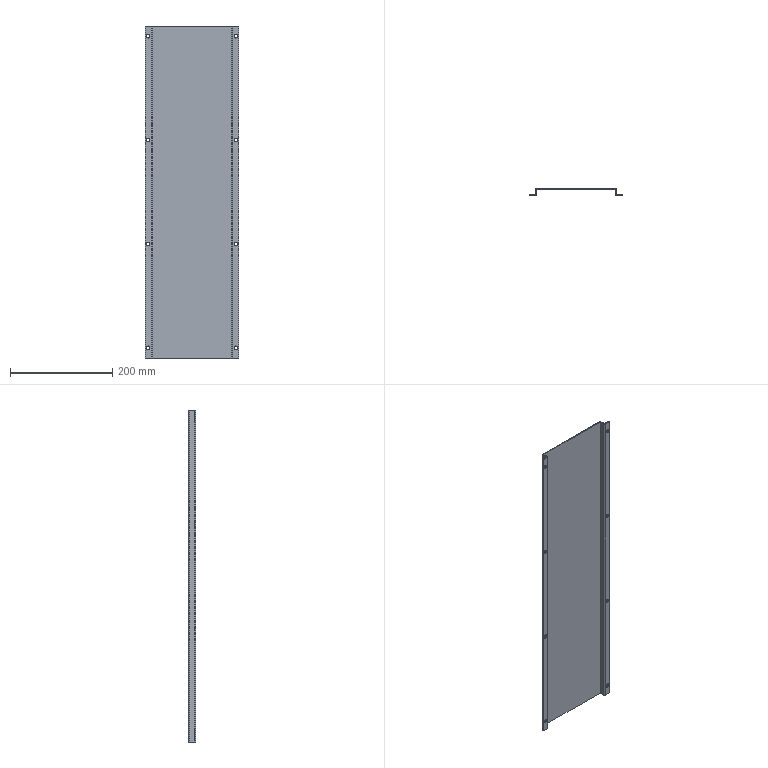Part | STEP file | Brake Resistor Plate | 1 solid | 38 faces | box 184 x 14 x 650 mm | volume 267329 mm3 | cylinder 24 | plane 14 | commonest cylinder face diameters 7 x16 0.2 x4 4.2 x4
STEP:
#1=CARTESIAN_POINT('',(61.034,19.025,633.5));
#2=VERTEX_POINT('',#1);
#3=CARTESIAN_POINT('',(61.034,19.025,626.5));
#4=VERTEX_POINT('',#3);
#5=CARTESIAN_POINT('',(61.034,19.025,630.));
#6=DIRECTION('',(0.,-1.,0.));
#7=DIRECTION('',(0.,0.,1.));
#8=AXIS2_PLACEMENT_3D('',#5,#6,#7);
#9=CIRCLE('',#8,3.5);
#10=EDGE_CURVE('',#2,#4,#9,.T.);
#11=ORIENTED_EDGE('',*,*,#10,.T.);
#12=CARTESIAN_POINT('',(61.034,21.025,626.5));
#13=VERTEX_POINT('',#12);
#14=CARTESIAN_POINT('',(61.034,11.025,626.5));
#15=DIRECTION('',(0.,1.,0.));
#16=VECTOR('',#15,1000.);
#17=LINE('',#14,#16);
#18=EDGE_CURVE('',#4,#13,#17,.T.);
#19=ORIENTED_EDGE('',*,*,#18,.T.);
#20=CARTESIAN_POINT('',(61.034,21.025,633.5));
#21=VERTEX_POINT('',#20);
#22=CARTESIAN_POINT('',(61.034,21.025,630.));
#23=DIRECTION('',(0.,-1.,0.));
#24=DIRECTION('',(0.,0.,1.));
#25=AXIS2_PLACEMENT_3D('',#22,#23,#24);
#26=CIRCLE('',#25,3.5);
#27=EDGE_CURVE('',#21,#13,#26,.T.);
#28=ORIENTED_EDGE('',*,*,#27,.F.);
#29=CARTESIAN_POINT('',(61.034,11.025,633.5));
#30=DIRECTION('',(0.,1.,0.));
#31=VECTOR('',#30,1000.);
#32=LINE('',#29,#31);
#33=EDGE_CURVE('',#2,#21,#32,.T.);
#34=ORIENTED_EDGE('',*,*,#33,.F.);
#35=EDGE_LOOP('',(#11,#19,#28,#34));
#36=FACE_OUTER_BOUND('',#35,.T.);
#37=CARTESIAN_POINT('',(61.034,11.025,630.));
#38=DIRECTION('',(0.,1.,0.));
#39=DIRECTION('',(0.,0.,1.));
#40=AXIS2_PLACEMENT_3D('',#37,#38,#39);
#41=CYLINDRICAL_SURFACE('',#40,3.5);
#42=ADVANCED_FACE('',(#36),#41,.F.);
#43=CARTESIAN_POINT('',(61.034,19.025,430.167));
#44=VERTEX_POINT('',#43);
#45=CARTESIAN_POINT('',(61.034,19.025,423.167));
#46=VERTEX_POINT('',#45);
#47=CARTESIAN_POINT('',(61.034,19.025,426.667));
#48=DIRECTION('',(0.,-1.,0.));
#49=DIRECTION('',(0.,0.,1.));
#50=AXIS2_PLACEMENT_3D('',#47,#48,#49);
#51=CIRCLE('',#50,3.5);
#52=EDGE_CURVE('',#44,#46,#51,.T.);
#53=ORIENTED_EDGE('',*,*,#52,.T.);
#54=CARTESIAN_POINT('',(61.034,21.025,423.167));
#55=VERTEX_POINT('',#54);
#56=CARTESIAN_POINT('',(61.034,11.025,423.167));
#57=DIRECTION('',(0.,1.,0.));
#58=VECTOR('',#57,1000.);
#59=LINE('',#56,#58);
#60=EDGE_CURVE('',#46,#55,#59,.T.);
#61=ORIENTED_EDGE('',*,*,#60,.T.);
#62=CARTESIAN_POINT('',(61.034,21.025,430.167));
#63=VERTEX_POINT('',#62);
#64=CARTESIAN_POINT('',(61.034,21.025,426.667));
#65=DIRECTION('',(0.,-1.,0.));
#66=DIRECTION('',(0.,0.,1.));
#67=AXIS2_PLACEMENT_3D('',#64,#65,#66);
#68=CIRCLE('',#67,3.5);
#69=EDGE_CURVE('',#63,#55,#68,.T.);
#70=ORIENTED_EDGE('',*,*,#69,.F.);
#71=CARTESIAN_POINT('',(61.034,11.025,430.167));
#72=DIRECTION('',(0.,1.,0.));
#73=VECTOR('',#72,1000.);
#74=LINE('',#71,#73);
#75=EDGE_CURVE('',#44,#63,#74,.T.);
#76=ORIENTED_EDGE('',*,*,#75,.F.);
#77=EDGE_LOOP('',(#53,#61,#70,#76));
#78=FACE_OUTER_BOUND('',#77,.T.);
#79=CARTESIAN_POINT('',(61.034,11.025,426.667));
#80=DIRECTION('',(0.,1.,0.));
#81=DIRECTION('',(0.,0.,1.));
#82=AXIS2_PLACEMENT_3D('',#79,#80,#81);
#83=CYLINDRICAL_SURFACE('',#82,3.5);
#84=ADVANCED_FACE('',(#78),#83,.F.);
#85=CARTESIAN_POINT('',(61.034,19.025,226.833));
#86=VERTEX_POINT('',#85);
#87=CARTESIAN_POINT('',(61.034,19.025,219.833));
#88=VERTEX_POINT('',#87);
#89=CARTESIAN_POINT('',(61.034,19.025,223.333));
#90=DIRECTION('',(0.,-1.,0.));
#91=DIRECTION('',(0.,0.,1.));
#92=AXIS2_PLACEMENT_3D('',#89,#90,#91);
#93=CIRCLE('',#92,3.5);
#94=EDGE_CURVE('',#86,#88,#93,.T.);
#95=ORIENTED_EDGE('',*,*,#94,.T.);
#96=CARTESIAN_POINT('',(61.034,21.025,219.833));
#97=VERTEX_POINT('',#96);
#98=CARTESIAN_POINT('',(61.034,11.025,219.833));
#99=DIRECTION('',(0.,1.,0.));
#100=VECTOR('',#99,1000.);
#101=LINE('',#98,#100);
#102=EDGE_CURVE('',#88,#97,#101,.T.);
#103=ORIENTED_EDGE('',*,*,#102,.T.);
#104=CARTESIAN_POINT('',(61.034,21.025,226.833));
#105=VERTEX_POINT('',#104);
#106=CARTESIAN_POINT('',(61.034,21.025,223.333));
#107=DIRECTION('',(0.,-1.,0.));
#108=DIRECTION('',(0.,0.,1.));
#109=AXIS2_PLACEMENT_3D('',#106,#107,#108);
#110=CIRCLE('',#109,3.5);
#111=EDGE_CURVE('',#105,#97,#110,.T.);
#112=ORIENTED_EDGE('',*,*,#111,.F.);
#113=CARTESIAN_POINT('',(61.034,11.025,226.833));
#114=DIRECTION('',(0.,1.,0.));
#115=VECTOR('',#114,1000.);
#116=LINE('',#113,#115);
#117=EDGE_CURVE('',#86,#105,#116,.T.);
#118=ORIENTED_EDGE('',*,*,#117,.F.);
#119=EDGE_LOOP('',(#95,#103,#112,#118));
#120=FACE_OUTER_BOUND('',#119,.T.);
#121=CARTESIAN_POINT('',(61.034,11.025,223.333));
#122=DIRECTION('',(0.,1.,0.));
#123=DIRECTION('',(0.,0.,1.));
#124=AXIS2_PLACEMENT_3D('',#121,#122,#123);
#125=CYLINDRICAL_SURFACE('',#124,3.5);
#126=ADVANCED_FACE('',(#120),#125,.F.);
#127=CARTESIAN_POINT('',(61.034,19.025,23.5));
#128=VERTEX_POINT('',#127);
#129=CARTESIAN_POINT('',(61.034,19.025,16.5));
#130=VERTEX_POINT('',#129);
#131=CARTESIAN_POINT('',(61.034,19.025,20.));
#132=DIRECTION('',(0.,-1.,0.));
#133=DIRECTION('',(0.,0.,1.));
#134=AXIS2_PLACEMENT_3D('',#131,#132,#133);
#135=CIRCLE('',#134,3.5);
#136=EDGE_CURVE('',#128,#130,#135,.T.);
#137=ORIENTED_EDGE('',*,*,#136,.T.);
#138=CARTESIAN_POINT('',(61.034,21.025,16.5));
#139=VERTEX_POINT('',#138);
#140=CARTESIAN_POINT('',(61.034,11.025,16.5));
#141=DIRECTION('',(0.,1.,0.));
#142=VECTOR('',#141,1000.);
#143=LINE('',#140,#142);
#144=EDGE_CURVE('',#130,#139,#143,.T.);
#145=ORIENTED_EDGE('',*,*,#144,.T.);
#146=CARTESIAN_POINT('',(61.034,21.025,23.5));
#147=VERTEX_POINT('',#146);
#148=CARTESIAN_POINT('',(61.034,21.025,20.));
#149=DIRECTION('',(0.,-1.,0.));
#150=DIRECTION('',(0.,0.,1.));
#151=AXIS2_PLACEMENT_3D('',#148,#149,#150);
#152=CIRCLE('',#151,3.5);
#153=EDGE_CURVE('',#147,#139,#152,.T.);
#154=ORIENTED_EDGE('',*,*,#153,.F.);
#155=CARTESIAN_POINT('',(61.034,11.025,23.5));
#156=DIRECTION('',(0.,1.,0.));
#157=VECTOR('',#156,1000.);
#158=LINE('',#155,#157);
#159=EDGE_CURVE('',#128,#147,#158,.T.);
#160=ORIENTED_EDGE('',*,*,#159,.F.);
#161=EDGE_LOOP('',(#137,#145,#154,#160));
#162=FACE_OUTER_BOUND('',#161,.T.);
#163=CARTESIAN_POINT('',(61.034,11.025,20.));
#164=DIRECTION('',(0.,1.,0.));
#165=DIRECTION('',(0.,0.,1.));
#166=AXIS2_PLACEMENT_3D('',#163,#164,#165);
#167=CYLINDRICAL_SURFACE('',#166,3.5);
#168=ADVANCED_FACE('',(#162),#167,.F.);
#169=CARTESIAN_POINT('',(-111.015,19.025,633.5));
#170=VERTEX_POINT('',#169);
#171=CARTESIAN_POINT('',(-111.015,19.025,626.5));
#172=VERTEX_POINT('',#171);
#173=CARTESIAN_POINT('',(-111.015,19.025,630.));
#174=DIRECTION('',(0.,-1.,0.));
#175=DIRECTION('',(0.,0.,1.));
#176=AXIS2_PLACEMENT_3D('',#173,#174,#175);
#177=CIRCLE('',#176,3.5);
#178=EDGE_CURVE('',#170,#172,#177,.T.);
#179=ORIENTED_EDGE('',*,*,#178,.T.);
#180=CARTESIAN_POINT('',(-111.015,21.025,626.5));
#181=VERTEX_POINT('',#180);
#182=CARTESIAN_POINT('',(-111.015,11.025,626.5));
#183=DIRECTION('',(0.,1.,0.));
#184=VECTOR('',#183,1000.);
#185=LINE('',#182,#184);
#186=EDGE_CURVE('',#172,#181,#185,.T.);
#187=ORIENTED_EDGE('',*,*,#186,.T.);
#188=CARTESIAN_POINT('',(-111.015,21.025,633.5));
#189=VERTEX_POINT('',#188);
#190=CARTESIAN_POINT('',(-111.015,21.025,630.));
#191=DIRECTION('',(0.,-1.,0.));
#192=DIRECTION('',(0.,0.,1.));
#193=AXIS2_PLACEMENT_3D('',#190,#191,#192);
#194=CIRCLE('',#193,3.5);
#195=EDGE_CURVE('',#189,#181,#194,.T.);
#196=ORIENTED_EDGE('',*,*,#195,.F.);
#197=CARTESIAN_POINT('',(-111.015,11.025,633.5));
#198=DIRECTION('',(0.,1.,0.));
#199=VECTOR('',#198,1000.);
#200=LINE('',#197,#199);
#201=EDGE_CURVE('',#170,#189,#200,.T.);
#202=ORIENTED_EDGE('',*,*,#201,.F.);
#203=EDGE_LOOP('',(#179,#187,#196,#202));
#204=FACE_OUTER_BOUND('',#203,.T.);
#205=CARTESIAN_POINT('',(-111.015,11.025,630.));
#206=DIRECTION('',(0.,1.,0.));
#207=DIRECTION('',(0.,0.,1.));
#208=AXIS2_PLACEMENT_3D('',#205,#206,#207);
#209=CYLINDRICAL_SURFACE('',#208,3.5);
#210=ADVANCED_FACE('',(#204),#209,.F.);
#211=CARTESIAN_POINT('',(-111.015,19.025,430.167));
#212=VERTEX_POINT('',#211);
#213=CARTESIAN_POINT('',(-111.015,19.025,423.167));
#214=VERTEX_POINT('',#213);
#215=CARTESIAN_POINT('',(-111.015,19.025,426.667));
#216=DIRECTION('',(0.,-1.,0.));
#217=DIRECTION('',(0.,0.,1.));
#218=AXIS2_PLACEMENT_3D('',#215,#216,#217);
#219=CIRCLE('',#218,3.5);
#220=EDGE_CURVE('',#212,#214,#219,.T.);
#221=ORIENTED_EDGE('',*,*,#220,.T.);
#222=CARTESIAN_POINT('',(-111.015,21.025,423.167));
#223=VERTEX_POINT('',#222);
#224=CARTESIAN_POINT('',(-111.015,11.025,423.167));
#225=DIRECTION('',(0.,1.,0.));
#226=VECTOR('',#225,1000.);
#227=LINE('',#224,#226);
#228=EDGE_CURVE('',#214,#223,#227,.T.);
#229=ORIENTED_EDGE('',*,*,#228,.T.);
#230=CARTESIAN_POINT('',(-111.015,21.025,430.167));
#231=VERTEX_POINT('',#230);
#232=CARTESIAN_POINT('',(-111.015,21.025,426.667));
#233=DIRECTION('',(0.,-1.,0.));
#234=DIRECTION('',(0.,0.,1.));
#235=AXIS2_PLACEMENT_3D('',#232,#233,#234);
#236=CIRCLE('',#235,3.5);
#237=EDGE_CURVE('',#231,#223,#236,.T.);
#238=ORIENTED_EDGE('',*,*,#237,.F.);
#239=CARTESIAN_POINT('',(-111.015,11.025,430.167));
#240=DIRECTION('',(0.,1.,0.));
#241=VECTOR('',#240,1000.);
#242=LINE('',#239,#241);
#243=EDGE_CURVE('',#212,#231,#242,.T.);
#244=ORIENTED_EDGE('',*,*,#243,.F.);
#245=EDGE_LOOP('',(#221,#229,#238,#244));
#246=FACE_OUTER_BOUND('',#245,.T.);
#247=CARTESIAN_POINT('',(-111.015,11.025,426.667));
#248=DIRECTION('',(0.,1.,0.));
#249=DIRECTION('',(0.,0.,1.));
#250=AXIS2_PLACEMENT_3D('',#247,#248,#249);
#251=CYLINDRICAL_SURFACE('',#250,3.5);
#252=ADVANCED_FACE('',(#246),#251,.F.);
#253=CARTESIAN_POINT('',(-111.015,19.025,226.833));
#254=VERTEX_POINT('',#253);
#255=CARTESIAN_POINT('',(-111.015,19.025,219.833));
#256=VERTEX_POINT('',#255);
#257=CARTESIAN_POINT('',(-111.015,19.025,223.333));
#258=DIRECTION('',(0.,-1.,0.));
#259=DIRECTION('',(0.,0.,1.));
#260=AXIS2_PLACEMENT_3D('',#257,#258,#259);
#261=CIRCLE('',#260,3.5);
#262=EDGE_CURVE('',#254,#256,#261,.T.);
#263=ORIENTED_EDGE('',*,*,#262,.T.);
#264=CARTESIAN_POINT('',(-111.015,21.025,219.833));
#265=VERTEX_POINT('',#264);
#266=CARTESIAN_POINT('',(-111.015,11.025,219.833));
#267=DIRECTION('',(0.,1.,0.));
#268=VECTOR('',#267,1000.);
#269=LINE('',#266,#268);
#270=EDGE_CURVE('',#256,#265,#269,.T.);
#271=ORIENTED_EDGE('',*,*,#270,.T.);
#272=CARTESIAN_POINT('',(-111.015,21.025,226.833));
#273=VERTEX_POINT('',#272);
#274=CARTESIAN_POINT('',(-111.015,21.025,223.333));
#275=DIRECTION('',(0.,-1.,0.));
#276=DIRECTION('',(0.,0.,1.));
#277=AXIS2_PLACEMENT_3D('',#274,#275,#276);
#278=CIRCLE('',#277,3.5);
#279=EDGE_CURVE('',#273,#265,#278,.T.);
#280=ORIENTED_EDGE('',*,*,#279,.F.);
#281=CARTESIAN_POINT('',(-111.015,11.025,226.833));
#282=DIRECTION('',(0.,1.,0.));
#283=VECTOR('',#282,1000.);
#284=LINE('',#281,#283);
#285=EDGE_CURVE('',#254,#273,#284,.T.);
#286=ORIENTED_EDGE('',*,*,#285,.F.);
#287=EDGE_LOOP('',(#263,#271,#280,#286));
#288=FACE_OUTER_BOUND('',#287,.T.);
#289=CARTESIAN_POINT('',(-111.015,11.025,223.333));
#290=DIRECTION('',(0.,1.,0.));
#291=DIRECTION('',(0.,0.,1.));
#292=AXIS2_PLACEMENT_3D('',#289,#290,#291);
#293=CYLINDRICAL_SURFACE('',#292,3.5);
#294=ADVANCED_FACE('',(#288),#293,.F.);
#295=CARTESIAN_POINT('',(-111.015,19.025,23.5));
#296=VERTEX_POINT('',#295);
#297=CARTESIAN_POINT('',(-111.015,19.025,16.5));
#298=VERTEX_POINT('',#297);
#299=CARTESIAN_POINT('',(-111.015,19.025,20.));
#300=DIRECTION('',(0.,-1.,0.));
#301=DIRECTION('',(0.,0.,1.));
#302=AXIS2_PLACEMENT_3D('',#299,#300,#301);
#303=CIRCLE('',#302,3.5);
#304=EDGE_CURVE('',#296,#298,#303,.T.);
#305=ORIENTED_EDGE('',*,*,#304,.T.);
#306=CARTESIAN_POINT('',(-111.015,21.025,16.5));
#307=VERTEX_POINT('',#306);
#308=CARTESIAN_POINT('',(-111.015,11.025,16.5));
#309=DIRECTION('',(0.,1.,0.));
#310=VECTOR('',#309,1000.);
#311=LINE('',#308,#310);
#312=EDGE_CURVE('',#298,#307,#311,.T.);
#313=ORIENTED_EDGE('',*,*,#312,.T.);
#314=CARTESIAN_POINT('',(-111.015,21.025,23.5));
#315=VERTEX_POINT('',#314);
#316=CARTESIAN_POINT('',(-111.015,21.025,20.));
#317=DIRECTION('',(0.,-1.,0.));
#318=DIRECTION('',(0.,0.,1.));
#319=AXIS2_PLACEMENT_3D('',#316,#317,#318);
#320=CIRCLE('',#319,3.5);
#321=EDGE_CURVE('',#315,#307,#320,.T.);
#322=ORIENTED_EDGE('',*,*,#321,.F.);
#323=CARTESIAN_POINT('',(-111.015,11.025,23.5));
#324=DIRECTION('',(0.,1.,0.));
#325=VECTOR('',#324,1000.);
#326=LINE('',#323,#325);
#327=EDGE_CURVE('',#296,#315,#326,.T.);
#328=ORIENTED_EDGE('',*,*,#327,.F.);
#329=EDGE_LOOP('',(#305,#313,#322,#328));
#330=FACE_OUTER_BOUND('',#329,.T.);
#331=CARTESIAN_POINT('',(-111.015,11.025,20.));
#332=DIRECTION('',(0.,1.,0.));
#333=DIRECTION('',(0.,0.,1.));
#334=AXIS2_PLACEMENT_3D('',#331,#332,#333);
#335=CYLINDRICAL_SURFACE('',#334,3.5);
#336=ADVANCED_FACE('',(#330),#335,.F.);
#337=CARTESIAN_POINT('',(52.934,31.025,650.));
#338=VERTEX_POINT('',#337);
#339=CARTESIAN_POINT('',(52.934,31.025,0.));
#340=VERTEX_POINT('',#339);
#341=CARTESIAN_POINT('',(52.934,31.025,650.));
#342=DIRECTION('',(0.,0.,-1.));
#343=VECTOR('',#342,1000.);
#344=LINE('',#341,#343);
#345=EDGE_CURVE('',#338,#340,#344,.T.);
#346=ORIENTED_EDGE('',*,*,#345,.F.);
#347=CARTESIAN_POINT('',(-102.866,31.025,650.));
#348=VERTEX_POINT('',#347);
#349=CARTESIAN_POINT('',(-104.966,31.025,650.));
#350=DIRECTION('',(1.,0.,0.));
#351=VECTOR('',#350,1000.);
#352=LINE('',#349,#351);
#353=EDGE_CURVE('',#348,#338,#352,.T.);
#354=ORIENTED_EDGE('',*,*,#353,.F.);
#355=CARTESIAN_POINT('',(-102.866,31.025,0.));
#356=VERTEX_POINT('',#355);
#357=CARTESIAN_POINT('',(-102.866,31.025,650.));
#358=DIRECTION('',(0.,0.,1.));
#359=VECTOR('',#358,1000.);
#360=LINE('',#357,#359);
#361=EDGE_CURVE('',#356,#348,#360,.T.);
#362=ORIENTED_EDGE('',*,*,#361,.F.);
#363=CARTESIAN_POINT('',(-104.966,31.025,0.));
#364=DIRECTION('',(-1.,0.,0.));
#365=VECTOR('',#364,1000.);
#366=LINE('',#363,#365);
#367=EDGE_CURVE('',#340,#356,#366,.T.);
#368=ORIENTED_EDGE('',*,*,#367,.F.);
#369=EDGE_LOOP('',(#346,#354,#362,#368));
#370=FACE_OUTER_BOUND('',#369,.T.);
#371=CARTESIAN_POINT('',(-104.966,31.025,650.));
#372=DIRECTION('',(0.,1.,0.));
#373=DIRECTION('',(0.,0.,1.));
#374=AXIS2_PLACEMENT_3D('',#371,#372,#373);
#375=PLANE('',#374);
#376=ADVANCED_FACE('',(#370),#375,.F.);
#377=ORIENTED_EDGE('',*,*,#367,.T.);
#378=CARTESIAN_POINT('',(-102.966,30.925,0.));
#379=VERTEX_POINT('',#378);
#380=CARTESIAN_POINT('',(-102.866,30.925,0.));
#381=DIRECTION('',(0.,0.,1.));
#382=DIRECTION('',(-1.,0.,0.));
#383=AXIS2_PLACEMENT_3D('',#380,#381,#382);
#384=CIRCLE('',#383,0.1);
#385=EDGE_CURVE('',#356,#379,#384,.T.);
#386=ORIENTED_EDGE('',*,*,#385,.T.);
#387=CARTESIAN_POINT('',(-102.966,21.125,0.));
#388=VERTEX_POINT('',#387);
#389=CARTESIAN_POINT('',(-102.966,21.025,0.));
#390=DIRECTION('',(0.,-1.,0.));
#391=VECTOR('',#390,1000.);
#392=LINE('',#389,#391);
#393=EDGE_CURVE('',#379,#388,#392,.T.);
#394=ORIENTED_EDGE('',*,*,#393,.T.);
#395=CARTESIAN_POINT('',(-105.066,19.025,0.));
#396=VERTEX_POINT('',#395);
#397=CARTESIAN_POINT('',(-105.066,21.125,0.));
#398=DIRECTION('',(0.,0.,1.));
#399=DIRECTION('',(-1.,0.,0.));
#400=AXIS2_PLACEMENT_3D('',#397,#398,#399);
#401=CIRCLE('',#400,2.1);
#402=EDGE_CURVE('',#396,#388,#401,.T.);
#403=ORIENTED_EDGE('',*,*,#402,.F.);
#404=CARTESIAN_POINT('',(-116.966,19.025,0.));
#405=VERTEX_POINT('',#404);
#406=CARTESIAN_POINT('',(-116.966,19.025,0.));
#407=DIRECTION('',(-1.,0.,0.));
#408=VECTOR('',#407,1000.);
#409=LINE('',#406,#408);
#410=EDGE_CURVE('',#396,#405,#409,.T.);
#411=ORIENTED_EDGE('',*,*,#410,.T.);
#412=CARTESIAN_POINT('',(-116.966,21.025,0.));
#413=VERTEX_POINT('',#412);
#414=CARTESIAN_POINT('',(-116.966,21.125,0.));
#415=DIRECTION('',(0.,1.,0.));
#416=VECTOR('',#415,1000.);
#417=LINE('',#414,#416);
#418=EDGE_CURVE('',#405,#413,#417,.T.);
#419=ORIENTED_EDGE('',*,*,#418,.T.);
#420=CARTESIAN_POINT('',(-105.066,21.025,0.));
#421=VERTEX_POINT('',#420);
#422=CARTESIAN_POINT('',(-102.966,21.025,0.));
#423=DIRECTION('',(1.,0.,0.));
#424=VECTOR('',#423,1000.);
#425=LINE('',#422,#424);
#426=EDGE_CURVE('',#413,#421,#425,.T.);
#427=ORIENTED_EDGE('',*,*,#426,.T.);
#428=CARTESIAN_POINT('',(-104.966,21.125,0.));
#429=VERTEX_POINT('',#428);
#430=CARTESIAN_POINT('',(-105.066,21.125,0.));
#431=DIRECTION('',(0.,0.,1.));
#432=DIRECTION('',(-1.,0.,0.));
#433=AXIS2_PLACEMENT_3D('',#430,#431,#432);
#434=CIRCLE('',#433,0.1);
#435=EDGE_CURVE('',#421,#429,#434,.T.);
#436=ORIENTED_EDGE('',*,*,#435,.T.);
#437=CARTESIAN_POINT('',(-104.966,30.925,0.));
#438=VERTEX_POINT('',#437);
#439=CARTESIAN_POINT('',(-104.966,31.025,0.));
#440=DIRECTION('',(0.,1.,0.));
#441=VECTOR('',#440,1000.);
#442=LINE('',#439,#441);
#443=EDGE_CURVE('',#429,#438,#442,.T.);
#444=ORIENTED_EDGE('',*,*,#443,.T.);
#445=CARTESIAN_POINT('',(-102.866,33.025,0.));
#446=VERTEX_POINT('',#445);
#447=CARTESIAN_POINT('',(-102.866,30.925,0.));
#448=DIRECTION('',(0.,0.,-1.));
#449=DIRECTION('',(-1.,0.,0.));
#450=AXIS2_PLACEMENT_3D('',#447,#448,#449);
#451=CIRCLE('',#450,2.1);
#452=EDGE_CURVE('',#438,#446,#451,.T.);
#453=ORIENTED_EDGE('',*,*,#452,.T.);
#454=CARTESIAN_POINT('',(52.934,33.025,0.));
#455=VERTEX_POINT('',#454);
#456=CARTESIAN_POINT('',(53.034,33.025,0.));
#457=DIRECTION('',(1.,0.,0.));
#458=VECTOR('',#457,1000.);
#459=LINE('',#456,#458);
#460=EDGE_CURVE('',#446,#455,#459,.T.);
#461=ORIENTED_EDGE('',*,*,#460,.T.);
#462=CARTESIAN_POINT('',(55.034,30.925,0.));
#463=VERTEX_POINT('',#462);
#464=CARTESIAN_POINT('',(52.934,30.925,0.));
#465=DIRECTION('',(0.,0.,-1.));
#466=DIRECTION('',(-1.,0.,0.));
#467=AXIS2_PLACEMENT_3D('',#464,#465,#466);
#468=CIRCLE('',#467,2.1);
#469=EDGE_CURVE('',#455,#463,#468,.T.);
#470=ORIENTED_EDGE('',*,*,#469,.T.);
#471=CARTESIAN_POINT('',(55.034,21.125,0.));
#472=VERTEX_POINT('',#471);
#473=CARTESIAN_POINT('',(55.034,19.025,0.));
#474=DIRECTION('',(0.,-1.,0.));
#475=VECTOR('',#474,1000.);
#476=LINE('',#473,#475);
#477=EDGE_CURVE('',#463,#472,#476,.T.);
#478=ORIENTED_EDGE('',*,*,#477,.T.);
#479=CARTESIAN_POINT('',(55.134,21.025,0.));
#480=VERTEX_POINT('',#479);
#481=CARTESIAN_POINT('',(55.134,21.125,0.));
#482=DIRECTION('',(0.,0.,1.));
#483=DIRECTION('',(-1.,0.,0.));
#484=AXIS2_PLACEMENT_3D('',#481,#482,#483);
#485=CIRCLE('',#484,0.1);
#486=EDGE_CURVE('',#472,#480,#485,.T.);
#487=ORIENTED_EDGE('',*,*,#486,.T.);
#488=CARTESIAN_POINT('',(67.034,21.025,0.));
#489=VERTEX_POINT('',#488);
#490=CARTESIAN_POINT('',(55.134,21.025,0.));
#491=DIRECTION('',(1.,0.,0.));
#492=VECTOR('',#491,1000.);
#493=LINE('',#490,#492);
#494=EDGE_CURVE('',#480,#489,#493,.T.);
#495=ORIENTED_EDGE('',*,*,#494,.T.);
#496=CARTESIAN_POINT('',(67.034,19.025,0.));
#497=VERTEX_POINT('',#496);
#498=CARTESIAN_POINT('',(67.034,21.125,0.));
#499=DIRECTION('',(0.,-1.,0.));
#500=VECTOR('',#499,1000.);
#501=LINE('',#498,#500);
#502=EDGE_CURVE('',#489,#497,#501,.T.);
#503=ORIENTED_EDGE('',*,*,#502,.T.);
#504=CARTESIAN_POINT('',(55.134,19.025,0.));
#505=VERTEX_POINT('',#504);
#506=CARTESIAN_POINT('',(55.034,19.025,0.));
#507=DIRECTION('',(-1.,0.,0.));
#508=VECTOR('',#507,1000.);
#509=LINE('',#506,#508);
#510=EDGE_CURVE('',#497,#505,#509,.T.);
#511=ORIENTED_EDGE('',*,*,#510,.T.);
#512=CARTESIAN_POINT('',(53.034,21.125,0.));
#513=VERTEX_POINT('',#512);
#514=CARTESIAN_POINT('',(55.134,21.125,0.));
#515=DIRECTION('',(0.,0.,1.));
#516=DIRECTION('',(-1.,0.,0.));
#517=AXIS2_PLACEMENT_3D('',#514,#515,#516);
#518=CIRCLE('',#517,2.1);
#519=EDGE_CURVE('',#513,#505,#518,.T.);
#520=ORIENTED_EDGE('',*,*,#519,.F.);
#521=CARTESIAN_POINT('',(53.034,30.925,0.));
#522=VERTEX_POINT('',#521);
#523=CARTESIAN_POINT('',(53.034,33.025,0.));
#524=DIRECTION('',(0.,1.,0.));
#525=VECTOR('',#524,1000.);
#526=LINE('',#523,#525);
#527=EDGE_CURVE('',#513,#522,#526,.T.);
#528=ORIENTED_EDGE('',*,*,#527,.T.);
#529=CARTESIAN_POINT('',(52.934,30.925,0.));
#530=DIRECTION('',(0.,0.,1.));
#531=DIRECTION('',(-1.,0.,0.));
#532=AXIS2_PLACEMENT_3D('',#529,#530,#531);
#533=CIRCLE('',#532,0.1);
#534=EDGE_CURVE('',#522,#340,#533,.T.);
#535=ORIENTED_EDGE('',*,*,#534,.T.);
#536=EDGE_LOOP('',(#377,#386,#394,#403,#411,#419,#427,#436,#444,#453,#461,#470,#478,#487,#495,#503,#511,#520,#528,#535));
#537=FACE_OUTER_BOUND('',#536,.T.);
#538=CARTESIAN_POINT('',(53.034,30.925,0.));
#539=DIRECTION('',(0.,0.,-1.));
#540=DIRECTION('',(-1.,0.,0.));
#541=AXIS2_PLACEMENT_3D('',#538,#539,#540);
#542=PLANE('',#541);
#543=ADVANCED_FACE('',(#537),#542,.T.);
#544=CARTESIAN_POINT('',(53.034,30.925,650.));
#545=VERTEX_POINT('',#544);
#546=CARTESIAN_POINT('',(53.034,30.925,650.));
#547=DIRECTION('',(0.,0.,-1.));
#548=VECTOR('',#547,1000.);
#549=LINE('',#546,#548);
#550=EDGE_CURVE('',#545,#522,#549,.T.);
#551=ORIENTED_EDGE('',*,*,#550,.F.);
#552=CARTESIAN_POINT('',(52.934,30.925,650.));
#553=DIRECTION('',(0.,0.,-1.));
#554=DIRECTION('',(-1.,0.,0.));
#555=AXIS2_PLACEMENT_3D('',#552,#553,#554);
#556=CIRCLE('',#555,0.1);
#557=EDGE_CURVE('',#338,#545,#556,.T.);
#558=ORIENTED_EDGE('',*,*,#557,.F.);
#559=ORIENTED_EDGE('',*,*,#345,.T.);
#560=ORIENTED_EDGE('',*,*,#534,.F.);
#561=EDGE_LOOP('',(#551,#558,#559,#560));
#562=FACE_OUTER_BOUND('',#561,.T.);
#563=CARTESIAN_POINT('',(52.934,30.925,650.));
#564=DIRECTION('',(0.,0.,-1.));
#565=DIRECTION('',(-1.,0.,0.));
#566=AXIS2_PLACEMENT_3D('',#563,#564,#565);
#567=CYLINDRICAL_SURFACE('',#566,0.1);
#568=ADVANCED_FACE('',(#562),#567,.F.);
#569=ORIENTED_EDGE('',*,*,#353,.T.);
#570=ORIENTED_EDGE('',*,*,#557,.T.);
#571=CARTESIAN_POINT('',(53.034,21.125,650.));
#572=VERTEX_POINT('',#571);
#573=CARTESIAN_POINT('',(53.034,33.025,650.));
#574=DIRECTION('',(0.,-1.,0.));
#575=VECTOR('',#574,1000.);
#576=LINE('',#573,#575);
#577=EDGE_CURVE('',#545,#572,#576,.T.);
#578=ORIENTED_EDGE('',*,*,#577,.T.);
#579=CARTESIAN_POINT('',(55.134,19.025,650.));
#580=VERTEX_POINT('',#579);
#581=CARTESIAN_POINT('',(55.134,21.125,650.));
#582=DIRECTION('',(0.,0.,-1.));
#583=DIRECTION('',(-1.,0.,0.));
#584=AXIS2_PLACEMENT_3D('',#581,#582,#583);
#585=CIRCLE('',#584,2.1);
#586=EDGE_CURVE('',#580,#572,#585,.T.);
#587=ORIENTED_EDGE('',*,*,#586,.F.);
#588=CARTESIAN_POINT('',(67.034,19.025,650.));
#589=VERTEX_POINT('',#588);
#590=CARTESIAN_POINT('',(55.034,19.025,650.));
#591=DIRECTION('',(1.,0.,0.));
#592=VECTOR('',#591,1000.);
#593=LINE('',#590,#592);
#594=EDGE_CURVE('',#580,#589,#593,.T.);
#595=ORIENTED_EDGE('',*,*,#594,.T.);
#596=CARTESIAN_POINT('',(67.034,21.025,650.));
#597=VERTEX_POINT('',#596);
#598=CARTESIAN_POINT('',(67.034,21.125,650.));
#599=DIRECTION('',(0.,1.,0.));
#600=VECTOR('',#599,1000.);
#601=LINE('',#598,#600);
#602=EDGE_CURVE('',#589,#597,#601,.T.);
#603=ORIENTED_EDGE('',*,*,#602,.T.);
#604=CARTESIAN_POINT('',(55.134,21.025,650.));
#605=VERTEX_POINT('',#604);
#606=CARTESIAN_POINT('',(53.034,21.025,650.));
#607=DIRECTION('',(-1.,0.,0.));
#608=VECTOR('',#607,1000.);
#609=LINE('',#606,#608);
#610=EDGE_CURVE('',#597,#605,#609,.T.);
#611=ORIENTED_EDGE('',*,*,#610,.T.);
#612=CARTESIAN_POINT('',(55.034,21.125,650.));
#613=VERTEX_POINT('',#612);
#614=CARTESIAN_POINT('',(55.134,21.125,650.));
#615=DIRECTION('',(0.,0.,-1.));
#616=DIRECTION('',(-1.,0.,0.));
#617=AXIS2_PLACEMENT_3D('',#614,#615,#616);
#618=CIRCLE('',#617,0.1);
#619=EDGE_CURVE('',#605,#613,#618,.T.);
#620=ORIENTED_EDGE('',*,*,#619,.T.);
#621=CARTESIAN_POINT('',(55.034,30.925,650.));
#622=VERTEX_POINT('',#621);
#623=CARTESIAN_POINT('',(55.034,31.025,650.));
#624=DIRECTION('',(0.,1.,0.));
#625=VECTOR('',#624,1000.);
#626=LINE('',#623,#625);
#627=EDGE_CURVE('',#613,#622,#626,.T.);
#628=ORIENTED_EDGE('',*,*,#627,.T.);
#629=CARTESIAN_POINT('',(52.934,33.025,650.));
#630=VERTEX_POINT('',#629);
#631=CARTESIAN_POINT('',(52.934,30.925,650.));
#632=DIRECTION('',(0.,0.,1.));
#633=DIRECTION('',(-1.,0.,0.));
#634=AXIS2_PLACEMENT_3D('',#631,#632,#633);
#635=CIRCLE('',#634,2.1);
#636=EDGE_CURVE('',#622,#630,#635,.T.);
#637=ORIENTED_EDGE('',*,*,#636,.T.);
#638=CARTESIAN_POINT('',(-102.866,33.025,650.));
#639=VERTEX_POINT('',#638);
#640=CARTESIAN_POINT('',(-102.966,33.025,650.));
#641=DIRECTION('',(-1.,0.,0.));
#642=VECTOR('',#641,1000.);
#643=LINE('',#640,#642);
#644=EDGE_CURVE('',#630,#639,#643,.T.);
#645=ORIENTED_EDGE('',*,*,#644,.T.);
#646=CARTESIAN_POINT('',(-104.966,30.925,650.));
#647=VERTEX_POINT('',#646);
#648=CARTESIAN_POINT('',(-102.866,30.925,650.));
#649=DIRECTION('',(0.,0.,1.));
#650=DIRECTION('',(-1.,0.,0.));
#651=AXIS2_PLACEMENT_3D('',#648,#649,#650);
#652=CIRCLE('',#651,2.1);
#653=EDGE_CURVE('',#639,#647,#652,.T.);
#654=ORIENTED_EDGE('',*,*,#653,.T.);
#655=CARTESIAN_POINT('',(-104.966,21.125,650.));
#656=VERTEX_POINT('',#655);
#657=CARTESIAN_POINT('',(-104.966,19.025,650.));
#658=DIRECTION('',(0.,-1.,0.));
#659=VECTOR('',#658,1000.);
#660=LINE('',#657,#659);
#661=EDGE_CURVE('',#647,#656,#660,.T.);
#662=ORIENTED_EDGE('',*,*,#661,.T.);
#663=CARTESIAN_POINT('',(-105.066,21.025,650.));
#664=VERTEX_POINT('',#663);
#665=CARTESIAN_POINT('',(-105.066,21.125,650.));
#666=DIRECTION('',(0.,0.,-1.));
#667=DIRECTION('',(-1.,0.,0.));
#668=AXIS2_PLACEMENT_3D('',#665,#666,#667);
#669=CIRCLE('',#668,0.1);
#670=EDGE_CURVE('',#656,#664,#669,.T.);
#671=ORIENTED_EDGE('',*,*,#670,.T.);
#672=CARTESIAN_POINT('',(-116.966,21.025,650.));
#673=VERTEX_POINT('',#672);
#674=CARTESIAN_POINT('',(55.134,21.025,650.));
#675=DIRECTION('',(1.,0.,0.));
#676=VECTOR('',#675,1000.);
#677=LINE('',#674,#676);
#678=EDGE_CURVE('',#673,#664,#677,.T.);
#679=ORIENTED_EDGE('',*,*,#678,.F.);
#680=CARTESIAN_POINT('',(-116.966,19.025,650.));
#681=VERTEX_POINT('',#680);
#682=CARTESIAN_POINT('',(-116.966,21.125,650.));
#683=DIRECTION('',(0.,1.,0.));
#684=VECTOR('',#683,1000.);
#685=LINE('',#682,#684);
#686=EDGE_CURVE('',#681,#673,#685,.T.);
#687=ORIENTED_EDGE('',*,*,#686,.F.);
#688=CARTESIAN_POINT('',(-105.066,19.025,650.));
#689=VERTEX_POINT('',#688);
#690=CARTESIAN_POINT('',(-116.966,19.025,650.));
#691=DIRECTION('',(1.,0.,0.));
#692=VECTOR('',#691,1000.);
#693=LINE('',#690,#692);
#694=EDGE_CURVE('',#681,#689,#693,.T.);
#695=ORIENTED_EDGE('',*,*,#694,.T.);
#696=CARTESIAN_POINT('',(-102.966,21.125,650.));
#697=VERTEX_POINT('',#696);
#698=CARTESIAN_POINT('',(-105.066,21.125,650.));
#699=DIRECTION('',(0.,0.,-1.));
#700=DIRECTION('',(-1.,0.,0.));
#701=AXIS2_PLACEMENT_3D('',#698,#699,#700);
#702=CIRCLE('',#701,2.1);
#703=EDGE_CURVE('',#697,#689,#702,.T.);
#704=ORIENTED_EDGE('',*,*,#703,.F.);
#705=CARTESIAN_POINT('',(-102.966,30.925,650.));
#706=VERTEX_POINT('',#705);
#707=CARTESIAN_POINT('',(-102.966,21.025,650.));
#708=DIRECTION('',(0.,1.,0.));
#709=VECTOR('',#708,1000.);
#710=LINE('',#707,#709);
#711=EDGE_CURVE('',#697,#706,#710,.T.);
#712=ORIENTED_EDGE('',*,*,#711,.T.);
#713=CARTESIAN_POINT('',(-102.866,30.925,650.));
#714=DIRECTION('',(0.,0.,-1.));
#715=DIRECTION('',(-1.,0.,0.));
#716=AXIS2_PLACEMENT_3D('',#713,#714,#715);
#717=CIRCLE('',#716,0.1);
#718=EDGE_CURVE('',#706,#348,#717,.T.);
#719=ORIENTED_EDGE('',*,*,#718,.T.);
#720=EDGE_LOOP('',(#569,#570,#578,#587,#595,#603,#611,#620,#628,#637,#645,#654,#662,#671,#679,#687,#695,#704,#712,#719));
#721=FACE_OUTER_BOUND('',#720,.T.);
#722=CARTESIAN_POINT('',(-102.966,30.925,650.));
#723=DIRECTION('',(0.,0.,1.));
#724=DIRECTION('',(1.,0.,0.));
#725=AXIS2_PLACEMENT_3D('',#722,#723,#724);
#726=PLANE('',#725);
#727=ADVANCED_FACE('',(#721),#726,.T.);
#728=ORIENTED_EDGE('',*,*,#361,.T.);
#729=ORIENTED_EDGE('',*,*,#718,.F.);
#730=CARTESIAN_POINT('',(-102.966,30.925,650.));
#731=DIRECTION('',(0.,0.,1.));
#732=VECTOR('',#731,1000.);
#733=LINE('',#730,#732);
#734=EDGE_CURVE('',#379,#706,#733,.T.);
#735=ORIENTED_EDGE('',*,*,#734,.F.);
#736=ORIENTED_EDGE('',*,*,#385,.F.);
#737=EDGE_LOOP('',(#728,#729,#735,#736));
#738=FACE_OUTER_BOUND('',#737,.T.);
#739=CARTESIAN_POINT('',(-102.866,30.925,650.));
#740=DIRECTION('',(0.,0.,-1.));
#741=DIRECTION('',(-1.,0.,0.));
#742=AXIS2_PLACEMENT_3D('',#739,#740,#741);
#743=CYLINDRICAL_SURFACE('',#742,0.1);
#744=ADVANCED_FACE('',(#738),#743,.F.);
#745=ORIENTED_EDGE('',*,*,#644,.F.);
#746=CARTESIAN_POINT('',(52.934,33.025,650.));
#747=DIRECTION('',(0.,0.,-1.));
#748=VECTOR('',#747,1000.);
#749=LINE('',#746,#748);
#750=EDGE_CURVE('',#630,#455,#749,.T.);
#751=ORIENTED_EDGE('',*,*,#750,.T.);
#752=ORIENTED_EDGE('',*,*,#460,.F.);
#753=CARTESIAN_POINT('',(-102.866,33.025,650.));
#754=DIRECTION('',(0.,0.,1.));
#755=VECTOR('',#754,1000.);
#756=LINE('',#753,#755);
#757=EDGE_CURVE('',#446,#639,#756,.T.);
#758=ORIENTED_EDGE('',*,*,#757,.T.);
#759=EDGE_LOOP('',(#745,#751,#752,#758));
#760=FACE_OUTER_BOUND('',#759,.T.);
#761=CARTESIAN_POINT('',(-104.966,33.025,650.));
#762=DIRECTION('',(0.,1.,0.));
#763=DIRECTION('',(0.,0.,1.));
#764=AXIS2_PLACEMENT_3D('',#761,#762,#763);
#765=PLANE('',#764);
#766=ADVANCED_FACE('',(#760),#765,.T.);
#767=CARTESIAN_POINT('',(53.034,21.125,650.));
#768=DIRECTION('',(0.,0.,-1.));
#769=VECTOR('',#768,1000.);
#770=LINE('',#767,#769);
#771=EDGE_CURVE('',#572,#513,#770,.T.);
#772=ORIENTED_EDGE('',*,*,#771,.F.);
#773=ORIENTED_EDGE('',*,*,#577,.F.);
#774=ORIENTED_EDGE('',*,*,#550,.T.);
#775=ORIENTED_EDGE('',*,*,#527,.F.);
#776=EDGE_LOOP('',(#772,#773,#774,#775));
#777=FACE_OUTER_BOUND('',#776,.T.);
#778=CARTESIAN_POINT('',(53.034,33.025,650.));
#779=DIRECTION('',(1.,0.,0.));
#780=DIRECTION('',(0.,1.,0.));
#781=AXIS2_PLACEMENT_3D('',#778,#779,#780);
#782=PLANE('',#781);
#783=ADVANCED_FACE('',(#777),#782,.F.);
#784=ORIENTED_EDGE('',*,*,#734,.T.);
#785=ORIENTED_EDGE('',*,*,#711,.F.);
#786=CARTESIAN_POINT('',(-102.966,21.125,650.));
#787=DIRECTION('',(0.,0.,1.));
#788=VECTOR('',#787,1000.);
#789=LINE('',#786,#788);
#790=EDGE_CURVE('',#388,#697,#789,.T.);
#791=ORIENTED_EDGE('',*,*,#790,.F.);
#792=ORIENTED_EDGE('',*,*,#393,.F.);
#793=EDGE_LOOP('',(#784,#785,#791,#792));
#794=FACE_OUTER_BOUND('',#793,.T.);
#795=CARTESIAN_POINT('',(-102.966,21.025,650.));
#796=DIRECTION('',(-1.,0.,0.));
#797=DIRECTION('',(0.,0.,1.));
#798=AXIS2_PLACEMENT_3D('',#795,#796,#797);
#799=PLANE('',#798);
#800=ADVANCED_FACE('',(#794),#799,.F.);
#801=ORIENTED_EDGE('',*,*,#653,.F.);
#802=ORIENTED_EDGE('',*,*,#757,.F.);
#803=ORIENTED_EDGE('',*,*,#452,.F.);
#804=CARTESIAN_POINT('',(-104.966,30.925,650.));
#805=DIRECTION('',(0.,0.,1.));
#806=VECTOR('',#805,1000.);
#807=LINE('',#804,#806);
#808=EDGE_CURVE('',#438,#647,#807,.T.);
#809=ORIENTED_EDGE('',*,*,#808,.T.);
#810=EDGE_LOOP('',(#801,#802,#803,#809));
#811=FACE_OUTER_BOUND('',#810,.T.);
#812=CARTESIAN_POINT('',(-102.866,30.925,650.));
#813=DIRECTION('',(0.,0.,-1.));
#814=DIRECTION('',(-1.,0.,0.));
#815=AXIS2_PLACEMENT_3D('',#812,#813,#814);
#816=CYLINDRICAL_SURFACE('',#815,2.1);
#817=ADVANCED_FACE('',(#811),#816,.T.);
#818=ORIENTED_EDGE('',*,*,#636,.F.);
#819=CARTESIAN_POINT('',(55.034,30.925,650.));
#820=DIRECTION('',(0.,0.,-1.));
#821=VECTOR('',#820,1000.);
#822=LINE('',#819,#821);
#823=EDGE_CURVE('',#622,#463,#822,.T.);
#824=ORIENTED_EDGE('',*,*,#823,.T.);
#825=ORIENTED_EDGE('',*,*,#469,.F.);
#826=ORIENTED_EDGE('',*,*,#750,.F.);
#827=EDGE_LOOP('',(#818,#824,#825,#826));
#828=FACE_OUTER_BOUND('',#827,.T.);
#829=CARTESIAN_POINT('',(52.934,30.925,650.));
#830=DIRECTION('',(0.,0.,-1.));
#831=DIRECTION('',(-1.,0.,0.));
#832=AXIS2_PLACEMENT_3D('',#829,#830,#831);
#833=CYLINDRICAL_SURFACE('',#832,2.1);
#834=ADVANCED_FACE('',(#828),#833,.T.);
#835=ORIENTED_EDGE('',*,*,#586,.T.);
#836=ORIENTED_EDGE('',*,*,#771,.T.);
#837=ORIENTED_EDGE('',*,*,#519,.T.);
#838=CARTESIAN_POINT('',(55.134,19.025,650.));
#839=DIRECTION('',(0.,0.,1.));
#840=VECTOR('',#839,1000.);
#841=LINE('',#838,#840);
#842=EDGE_CURVE('',#505,#580,#841,.T.);
#843=ORIENTED_EDGE('',*,*,#842,.T.);
#844=EDGE_LOOP('',(#835,#836,#837,#843));
#845=FACE_OUTER_BOUND('',#844,.T.);
#846=CARTESIAN_POINT('',(55.134,21.125,650.));
#847=DIRECTION('',(0.,0.,-1.));
#848=DIRECTION('',(-1.,0.,0.));
#849=AXIS2_PLACEMENT_3D('',#846,#847,#848);
#850=CYLINDRICAL_SURFACE('',#849,2.1);
#851=ADVANCED_FACE('',(#845),#850,.T.);
#852=ORIENTED_EDGE('',*,*,#703,.T.);
#853=CARTESIAN_POINT('',(-105.066,19.025,650.));
#854=DIRECTION('',(0.,0.,-1.));
#855=VECTOR('',#854,1000.);
#856=LINE('',#853,#855);
#857=EDGE_CURVE('',#689,#396,#856,.T.);
#858=ORIENTED_EDGE('',*,*,#857,.T.);
#859=ORIENTED_EDGE('',*,*,#402,.T.);
#860=ORIENTED_EDGE('',*,*,#790,.T.);
#861=EDGE_LOOP('',(#852,#858,#859,#860));
#862=FACE_OUTER_BOUND('',#861,.T.);
#863=CARTESIAN_POINT('',(-105.066,21.125,650.));
#864=DIRECTION('',(0.,0.,-1.));
#865=DIRECTION('',(-1.,0.,0.));
#866=AXIS2_PLACEMENT_3D('',#863,#864,#865);
#867=CYLINDRICAL_SURFACE('',#866,2.1);
#868=ADVANCED_FACE('',(#862),#867,.T.);
#869=ORIENTED_EDGE('',*,*,#661,.F.);
#870=ORIENTED_EDGE('',*,*,#808,.F.);
#871=ORIENTED_EDGE('',*,*,#443,.F.);
#872=CARTESIAN_POINT('',(-104.966,21.125,650.));
#873=DIRECTION('',(0.,0.,1.));
#874=VECTOR('',#873,1000.);
#875=LINE('',#872,#874);
#876=EDGE_CURVE('',#429,#656,#875,.T.);
#877=ORIENTED_EDGE('',*,*,#876,.T.);
#878=EDGE_LOOP('',(#869,#870,#871,#877));
#879=FACE_OUTER_BOUND('',#878,.T.);
#880=CARTESIAN_POINT('',(-104.966,21.025,650.));
#881=DIRECTION('',(-1.,0.,0.));
#882=DIRECTION('',(0.,0.,1.));
#883=AXIS2_PLACEMENT_3D('',#880,#881,#882);
#884=PLANE('',#883);
#885=ADVANCED_FACE('',(#879),#884,.T.);
#886=ORIENTED_EDGE('',*,*,#627,.F.);
#887=CARTESIAN_POINT('',(55.034,21.125,650.));
#888=DIRECTION('',(0.,0.,-1.));
#889=VECTOR('',#888,1000.);
#890=LINE('',#887,#889);
#891=EDGE_CURVE('',#613,#472,#890,.T.);
#892=ORIENTED_EDGE('',*,*,#891,.T.);
#893=ORIENTED_EDGE('',*,*,#477,.F.);
#894=ORIENTED_EDGE('',*,*,#823,.F.);
#895=EDGE_LOOP('',(#886,#892,#893,#894));
#896=FACE_OUTER_BOUND('',#895,.T.);
#897=CARTESIAN_POINT('',(55.034,33.025,650.));
#898=DIRECTION('',(1.,0.,0.));
#899=DIRECTION('',(0.,1.,0.));
#900=AXIS2_PLACEMENT_3D('',#897,#898,#899);
#901=PLANE('',#900);
#902=ADVANCED_FACE('',(#896),#901,.T.);
#903=CARTESIAN_POINT('',(67.034,19.025,650.));
#904=DIRECTION('',(0.,0.,-1.));
#905=VECTOR('',#904,1000.);
#906=LINE('',#903,#905);
#907=EDGE_CURVE('',#589,#497,#906,.T.);
#908=ORIENTED_EDGE('',*,*,#907,.F.);
#909=ORIENTED_EDGE('',*,*,#594,.F.);
#910=ORIENTED_EDGE('',*,*,#842,.F.);
#911=ORIENTED_EDGE('',*,*,#510,.F.);
#912=EDGE_LOOP('',(#908,#909,#910,#911));
#913=FACE_OUTER_BOUND('',#912,.T.);
#914=ORIENTED_EDGE('',*,*,#10,.F.);
#915=CARTESIAN_POINT('',(61.034,19.025,630.));
#916=DIRECTION('',(0.,-1.,0.));
#917=DIRECTION('',(0.,0.,1.));
#918=AXIS2_PLACEMENT_3D('',#915,#916,#917);
#919=CIRCLE('',#918,3.5);
#920=EDGE_CURVE('',#4,#2,#919,.T.);
#921=ORIENTED_EDGE('',*,*,#920,.F.);
#922=EDGE_LOOP('',(#914,#921));
#923=FACE_BOUND('',#922,.T.);
#924=ORIENTED_EDGE('',*,*,#52,.F.);
#925=CARTESIAN_POINT('',(61.034,19.025,426.667));
#926=DIRECTION('',(0.,-1.,0.));
#927=DIRECTION('',(0.,0.,1.));
#928=AXIS2_PLACEMENT_3D('',#925,#926,#927);
#929=CIRCLE('',#928,3.5);
#930=EDGE_CURVE('',#46,#44,#929,.T.);
#931=ORIENTED_EDGE('',*,*,#930,.F.);
#932=EDGE_LOOP('',(#924,#931));
#933=FACE_BOUND('',#932,.T.);
#934=ORIENTED_EDGE('',*,*,#94,.F.);
#935=CARTESIAN_POINT('',(61.034,19.025,223.333));
#936=DIRECTION('',(0.,-1.,0.));
#937=DIRECTION('',(0.,0.,1.));
#938=AXIS2_PLACEMENT_3D('',#935,#936,#937);
#939=CIRCLE('',#938,3.5);
#940=EDGE_CURVE('',#88,#86,#939,.T.);
#941=ORIENTED_EDGE('',*,*,#940,.F.);
#942=EDGE_LOOP('',(#934,#941));
#943=FACE_BOUND('',#942,.T.);
#944=ORIENTED_EDGE('',*,*,#136,.F.);
#945=CARTESIAN_POINT('',(61.034,19.025,20.));
#946=DIRECTION('',(0.,-1.,0.));
#947=DIRECTION('',(0.,0.,1.));
#948=AXIS2_PLACEMENT_3D('',#945,#946,#947);
#949=CIRCLE('',#948,3.5);
#950=EDGE_CURVE('',#130,#128,#949,.T.);
#951=ORIENTED_EDGE('',*,*,#950,.F.);
#952=EDGE_LOOP('',(#944,#951));
#953=FACE_BOUND('',#952,.T.);
#954=CARTESIAN_POINT('',(55.034,19.025,650.));
#955=DIRECTION('',(0.,1.,0.));
#956=DIRECTION('',(0.,0.,1.));
#957=AXIS2_PLACEMENT_3D('',#954,#955,#956);
#958=PLANE('',#957);
#959=ADVANCED_FACE('',(#913,#923,#933,#943,#953),#958,.F.);
#960=ORIENTED_EDGE('',*,*,#857,.F.);
#961=ORIENTED_EDGE('',*,*,#694,.F.);
#962=CARTESIAN_POINT('',(-116.966,19.025,650.));
#963=DIRECTION('',(0.,0.,1.));
#964=VECTOR('',#963,1000.);
#965=LINE('',#962,#964);
#966=EDGE_CURVE('',#405,#681,#965,.T.);
#967=ORIENTED_EDGE('',*,*,#966,.F.);
#968=ORIENTED_EDGE('',*,*,#410,.F.);
#969=EDGE_LOOP('',(#960,#961,#967,#968));
#970=FACE_OUTER_BOUND('',#969,.T.);
#971=ORIENTED_EDGE('',*,*,#178,.F.);
#972=CARTESIAN_POINT('',(-111.015,19.025,630.));
#973=DIRECTION('',(0.,-1.,0.));
#974=DIRECTION('',(0.,0.,1.));
#975=AXIS2_PLACEMENT_3D('',#972,#973,#974);
#976=CIRCLE('',#975,3.5);
#977=EDGE_CURVE('',#172,#170,#976,.T.);
#978=ORIENTED_EDGE('',*,*,#977,.F.);
#979=EDGE_LOOP('',(#971,#978));
#980=FACE_BOUND('',#979,.T.);
#981=ORIENTED_EDGE('',*,*,#220,.F.);
#982=CARTESIAN_POINT('',(-111.015,19.025,426.667));
#983=DIRECTION('',(0.,-1.,0.));
#984=DIRECTION('',(0.,0.,1.));
#985=AXIS2_PLACEMENT_3D('',#982,#983,#984);
#986=CIRCLE('',#985,3.5);
#987=EDGE_CURVE('',#214,#212,#986,.T.);
#988=ORIENTED_EDGE('',*,*,#987,.F.);
#989=EDGE_LOOP('',(#981,#988));
#990=FACE_BOUND('',#989,.T.);
#991=ORIENTED_EDGE('',*,*,#262,.F.);
#992=CARTESIAN_POINT('',(-111.015,19.025,223.333));
#993=DIRECTION('',(0.,-1.,0.));
#994=DIRECTION('',(0.,0.,1.));
#995=AXIS2_PLACEMENT_3D('',#992,#993,#994);
#996=CIRCLE('',#995,3.5);
#997=EDGE_CURVE('',#256,#254,#996,.T.);
#998=ORIENTED_EDGE('',*,*,#997,.F.);
#999=EDGE_LOOP('',(#991,#998));
#1000=FACE_BOUND('',#999,.T.);
#1001=ORIENTED_EDGE('',*,*,#304,.F.);
#1002=CARTESIAN_POINT('',(-111.015,19.025,20.));
#1003=DIRECTION('',(0.,-1.,0.));
#1004=DIRECTION('',(0.,0.,1.));
#1005=AXIS2_PLACEMENT_3D('',#1002,#1003,#1004);
#1006=CIRCLE('',#1005,3.5);
#1007=EDGE_CURVE('',#298,#296,#1006,.T.);
#1008=ORIENTED_EDGE('',*,*,#1007,.F.);
#1009=EDGE_LOOP('',(#1001,#1008));
#1010=FACE_BOUND('',#1009,.T.);
#1011=CARTESIAN_POINT('',(-116.966,19.025,650.));
#1012=DIRECTION('',(0.,1.,0.));
#1013=DIRECTION('',(-1.,0.,0.));
#1014=AXIS2_PLACEMENT_3D('',#1011,#1012,#1013);
#1015=PLANE('',#1014);
#1016=ADVANCED_FACE('',(#970,#980,#990,#1000,#1010),#1015,.F.);
#1017=CARTESIAN_POINT('',(-105.066,21.025,650.));
#1018=DIRECTION('',(0.,0.,-1.));
#1019=VECTOR('',#1018,1000.);
#1020=LINE('',#1017,#1019);
#1021=EDGE_CURVE('',#664,#421,#1020,.T.);
#1022=ORIENTED_EDGE('',*,*,#1021,.F.);
#1023=ORIENTED_EDGE('',*,*,#670,.F.);
#1024=ORIENTED_EDGE('',*,*,#876,.F.);
#1025=ORIENTED_EDGE('',*,*,#435,.F.);
#1026=EDGE_LOOP('',(#1022,#1023,#1024,#1025));
#1027=FACE_OUTER_BOUND('',#1026,.T.);
#1028=CARTESIAN_POINT('',(-105.066,21.125,650.));
#1029=DIRECTION('',(0.,0.,-1.));
#1030=DIRECTION('',(-1.,0.,0.));
#1031=AXIS2_PLACEMENT_3D('',#1028,#1029,#1030);
#1032=CYLINDRICAL_SURFACE('',#1031,0.1);
#1033=ADVANCED_FACE('',(#1027),#1032,.F.);
#1034=ORIENTED_EDGE('',*,*,#891,.F.);
#1035=ORIENTED_EDGE('',*,*,#619,.F.);
#1036=CARTESIAN_POINT('',(55.134,21.025,650.));
#1037=DIRECTION('',(0.,0.,1.));
#1038=VECTOR('',#1037,1000.);
#1039=LINE('',#1036,#1038);
#1040=EDGE_CURVE('',#480,#605,#1039,.T.);
#1041=ORIENTED_EDGE('',*,*,#1040,.F.);
#1042=ORIENTED_EDGE('',*,*,#486,.F.);
#1043=EDGE_LOOP('',(#1034,#1035,#1041,#1042));
#1044=FACE_OUTER_BOUND('',#1043,.T.);
#1045=CARTESIAN_POINT('',(55.134,21.125,650.));
#1046=DIRECTION('',(0.,0.,-1.));
#1047=DIRECTION('',(-1.,0.,0.));
#1048=AXIS2_PLACEMENT_3D('',#1045,#1046,#1047);
#1049=CYLINDRICAL_SURFACE('',#1048,0.1);
#1050=ADVANCED_FACE('',(#1044),#1049,.F.);
#1051=ORIENTED_EDGE('',*,*,#602,.F.);
#1052=ORIENTED_EDGE('',*,*,#907,.T.);
#1053=ORIENTED_EDGE('',*,*,#502,.F.);
#1054=CARTESIAN_POINT('',(67.034,21.025,650.));
#1055=DIRECTION('',(0.,0.,1.));
#1056=VECTOR('',#1055,1000.);
#1057=LINE('',#1054,#1056);
#1058=EDGE_CURVE('',#489,#597,#1057,.T.);
#1059=ORIENTED_EDGE('',*,*,#1058,.T.);
#1060=EDGE_LOOP('',(#1051,#1052,#1053,#1059));
#1061=FACE_OUTER_BOUND('',#1060,.T.);
#1062=CARTESIAN_POINT('',(67.034,21.025,650.));
#1063=DIRECTION('',(1.,0.,0.));
#1064=DIRECTION('',(0.,0.,-1.));
#1065=AXIS2_PLACEMENT_3D('',#1062,#1063,#1064);
#1066=PLANE('',#1065);
#1067=ADVANCED_FACE('',(#1061),#1066,.T.);
#1068=ORIENTED_EDGE('',*,*,#18,.F.);
#1069=ORIENTED_EDGE('',*,*,#920,.T.);
#1070=ORIENTED_EDGE('',*,*,#33,.T.);
#1071=CARTESIAN_POINT('',(61.034,21.025,630.));
#1072=DIRECTION('',(0.,-1.,0.));
#1073=DIRECTION('',(0.,0.,1.));
#1074=AXIS2_PLACEMENT_3D('',#1071,#1072,#1073);
#1075=CIRCLE('',#1074,3.5);
#1076=EDGE_CURVE('',#13,#21,#1075,.T.);
#1077=ORIENTED_EDGE('',*,*,#1076,.F.);
#1078=EDGE_LOOP('',(#1068,#1069,#1070,#1077));
#1079=FACE_OUTER_BOUND('',#1078,.T.);
#1080=CARTESIAN_POINT('',(61.034,11.025,630.));
#1081=DIRECTION('',(0.,1.,0.));
#1082=DIRECTION('',(0.,0.,1.));
#1083=AXIS2_PLACEMENT_3D('',#1080,#1081,#1082);
#1084=CYLINDRICAL_SURFACE('',#1083,3.5);
#1085=ADVANCED_FACE('',(#1079),#1084,.F.);
#1086=ORIENTED_EDGE('',*,*,#60,.F.);
#1087=ORIENTED_EDGE('',*,*,#930,.T.);
#1088=ORIENTED_EDGE('',*,*,#75,.T.);
#1089=CARTESIAN_POINT('',(61.034,21.025,426.667));
#1090=DIRECTION('',(0.,-1.,0.));
#1091=DIRECTION('',(0.,0.,1.));
#1092=AXIS2_PLACEMENT_3D('',#1089,#1090,#1091);
#1093=CIRCLE('',#1092,3.5);
#1094=EDGE_CURVE('',#55,#63,#1093,.T.);
#1095=ORIENTED_EDGE('',*,*,#1094,.F.);
#1096=EDGE_LOOP('',(#1086,#1087,#1088,#1095));
#1097=FACE_OUTER_BOUND('',#1096,.T.);
#1098=CARTESIAN_POINT('',(61.034,11.025,426.667));
#1099=DIRECTION('',(0.,1.,0.));
#1100=DIRECTION('',(0.,0.,1.));
#1101=AXIS2_PLACEMENT_3D('',#1098,#1099,#1100);
#1102=CYLINDRICAL_SURFACE('',#1101,3.5);
#1103=ADVANCED_FACE('',(#1097),#1102,.F.);
#1104=ORIENTED_EDGE('',*,*,#102,.F.);
#1105=ORIENTED_EDGE('',*,*,#940,.T.);
#1106=ORIENTED_EDGE('',*,*,#117,.T.);
#1107=CARTESIAN_POINT('',(61.034,21.025,223.333));
#1108=DIRECTION('',(0.,-1.,0.));
#1109=DIRECTION('',(0.,0.,1.));
#1110=AXIS2_PLACEMENT_3D('',#1107,#1108,#1109);
#1111=CIRCLE('',#1110,3.5);
#1112=EDGE_CURVE('',#97,#105,#1111,.T.);
#1113=ORIENTED_EDGE('',*,*,#1112,.F.);
#1114=EDGE_LOOP('',(#1104,#1105,#1106,#1113));
#1115=FACE_OUTER_BOUND('',#1114,.T.);
#1116=CARTESIAN_POINT('',(61.034,11.025,223.333));
#1117=DIRECTION('',(0.,1.,0.));
#1118=DIRECTION('',(0.,0.,1.));
#1119=AXIS2_PLACEMENT_3D('',#1116,#1117,#1118);
#1120=CYLINDRICAL_SURFACE('',#1119,3.5);
#1121=ADVANCED_FACE('',(#1115),#1120,.F.);
#1122=ORIENTED_EDGE('',*,*,#144,.F.);
#1123=ORIENTED_EDGE('',*,*,#950,.T.);
#1124=ORIENTED_EDGE('',*,*,#159,.T.);
#1125=CARTESIAN_POINT('',(61.034,21.025,20.));
#1126=DIRECTION('',(0.,-1.,0.));
#1127=DIRECTION('',(0.,0.,1.));
#1128=AXIS2_PLACEMENT_3D('',#1125,#1126,#1127);
#1129=CIRCLE('',#1128,3.5);
#1130=EDGE_CURVE('',#139,#147,#1129,.T.);
#1131=ORIENTED_EDGE('',*,*,#1130,.F.);
#1132=EDGE_LOOP('',(#1122,#1123,#1124,#1131));
#1133=FACE_OUTER_BOUND('',#1132,.T.);
#1134=CARTESIAN_POINT('',(61.034,11.025,20.));
#1135=DIRECTION('',(0.,1.,0.));
#1136=DIRECTION('',(0.,0.,1.));
#1137=AXIS2_PLACEMENT_3D('',#1134,#1135,#1136);
#1138=CYLINDRICAL_SURFACE('',#1137,3.5);
#1139=ADVANCED_FACE('',(#1133),#1138,.F.);
#1140=ORIENTED_EDGE('',*,*,#686,.T.);
#1141=CARTESIAN_POINT('',(-116.966,21.025,650.));
#1142=DIRECTION('',(0.,0.,-1.));
#1143=VECTOR('',#1142,1000.);
#1144=LINE('',#1141,#1143);
#1145=EDGE_CURVE('',#673,#413,#1144,.T.);
#1146=ORIENTED_EDGE('',*,*,#1145,.T.);
#1147=ORIENTED_EDGE('',*,*,#418,.F.);
#1148=ORIENTED_EDGE('',*,*,#966,.T.);
#1149=EDGE_LOOP('',(#1140,#1146,#1147,#1148));
#1150=FACE_OUTER_BOUND('',#1149,.T.);
#1151=CARTESIAN_POINT('',(-116.966,19.025,650.));
#1152=DIRECTION('',(-1.,0.,0.));
#1153=DIRECTION('',(0.,0.,1.));
#1154=AXIS2_PLACEMENT_3D('',#1151,#1152,#1153);
#1155=PLANE('',#1154);
#1156=ADVANCED_FACE('',(#1150),#1155,.T.);
#1157=ORIENTED_EDGE('',*,*,#186,.F.);
#1158=ORIENTED_EDGE('',*,*,#977,.T.);
#1159=ORIENTED_EDGE('',*,*,#201,.T.);
#1160=CARTESIAN_POINT('',(-111.015,21.025,630.));
#1161=DIRECTION('',(0.,-1.,0.));
#1162=DIRECTION('',(0.,0.,1.));
#1163=AXIS2_PLACEMENT_3D('',#1160,#1161,#1162);
#1164=CIRCLE('',#1163,3.5);
#1165=EDGE_CURVE('',#181,#189,#1164,.T.);
#1166=ORIENTED_EDGE('',*,*,#1165,.F.);
#1167=EDGE_LOOP('',(#1157,#1158,#1159,#1166));
#1168=FACE_OUTER_BOUND('',#1167,.T.);
#1169=CARTESIAN_POINT('',(-111.015,11.025,630.));
#1170=DIRECTION('',(0.,1.,0.));
#1171=DIRECTION('',(0.,0.,1.));
#1172=AXIS2_PLACEMENT_3D('',#1169,#1170,#1171);
#1173=CYLINDRICAL_SURFACE('',#1172,3.5);
#1174=ADVANCED_FACE('',(#1168),#1173,.F.);
#1175=ORIENTED_EDGE('',*,*,#228,.F.);
#1176=ORIENTED_EDGE('',*,*,#987,.T.);
#1177=ORIENTED_EDGE('',*,*,#243,.T.);
#1178=CARTESIAN_POINT('',(-111.015,21.025,426.667));
#1179=DIRECTION('',(0.,-1.,0.));
#1180=DIRECTION('',(0.,0.,1.));
#1181=AXIS2_PLACEMENT_3D('',#1178,#1179,#1180);
#1182=CIRCLE('',#1181,3.5);
#1183=EDGE_CURVE('',#223,#231,#1182,.T.);
#1184=ORIENTED_EDGE('',*,*,#1183,.F.);
#1185=EDGE_LOOP('',(#1175,#1176,#1177,#1184));
#1186=FACE_OUTER_BOUND('',#1185,.T.);
#1187=CARTESIAN_POINT('',(-111.015,11.025,426.667));
#1188=DIRECTION('',(0.,1.,0.));
#1189=DIRECTION('',(0.,0.,1.));
#1190=AXIS2_PLACEMENT_3D('',#1187,#1188,#1189);
#1191=CYLINDRICAL_SURFACE('',#1190,3.5);
#1192=ADVANCED_FACE('',(#1186),#1191,.F.);
#1193=ORIENTED_EDGE('',*,*,#270,.F.);
#1194=ORIENTED_EDGE('',*,*,#997,.T.);
#1195=ORIENTED_EDGE('',*,*,#285,.T.);
#1196=CARTESIAN_POINT('',(-111.015,21.025,223.333));
#1197=DIRECTION('',(0.,-1.,0.));
#1198=DIRECTION('',(0.,0.,1.));
#1199=AXIS2_PLACEMENT_3D('',#1196,#1197,#1198);
#1200=CIRCLE('',#1199,3.5);
#1201=EDGE_CURVE('',#265,#273,#1200,.T.);
#1202=ORIENTED_EDGE('',*,*,#1201,.F.);
#1203=EDGE_LOOP('',(#1193,#1194,#1195,#1202));
#1204=FACE_OUTER_BOUND('',#1203,.T.);
#1205=CARTESIAN_POINT('',(-111.015,11.025,223.333));
#1206=DIRECTION('',(0.,1.,0.));
#1207=DIRECTION('',(0.,0.,1.));
#1208=AXIS2_PLACEMENT_3D('',#1205,#1206,#1207);
#1209=CYLINDRICAL_SURFACE('',#1208,3.5);
#1210=ADVANCED_FACE('',(#1204),#1209,.F.);
#1211=ORIENTED_EDGE('',*,*,#312,.F.);
#1212=ORIENTED_EDGE('',*,*,#1007,.T.);
#1213=ORIENTED_EDGE('',*,*,#327,.T.);
#1214=CARTESIAN_POINT('',(-111.015,21.025,20.));
#1215=DIRECTION('',(0.,-1.,0.));
#1216=DIRECTION('',(0.,0.,1.));
#1217=AXIS2_PLACEMENT_3D('',#1214,#1215,#1216);
#1218=CIRCLE('',#1217,3.5);
#1219=EDGE_CURVE('',#307,#315,#1218,.T.);
#1220=ORIENTED_EDGE('',*,*,#1219,.F.);
#1221=EDGE_LOOP('',(#1211,#1212,#1213,#1220));
#1222=FACE_OUTER_BOUND('',#1221,.T.);
#1223=CARTESIAN_POINT('',(-111.015,11.025,20.));
#1224=DIRECTION('',(0.,1.,0.));
#1225=DIRECTION('',(0.,0.,1.));
#1226=AXIS2_PLACEMENT_3D('',#1223,#1224,#1225);
#1227=CYLINDRICAL_SURFACE('',#1226,3.5);
#1228=ADVANCED_FACE('',(#1222),#1227,.F.);
#1229=ORIENTED_EDGE('',*,*,#678,.T.);
#1230=ORIENTED_EDGE('',*,*,#1021,.T.);
#1231=ORIENTED_EDGE('',*,*,#426,.F.);
#1232=ORIENTED_EDGE('',*,*,#1145,.F.);
#1233=EDGE_LOOP('',(#1229,#1230,#1231,#1232));
#1234=FACE_OUTER_BOUND('',#1233,.T.);
#1235=ORIENTED_EDGE('',*,*,#195,.T.);
#1236=ORIENTED_EDGE('',*,*,#1165,.T.);
#1237=EDGE_LOOP('',(#1235,#1236));
#1238=FACE_BOUND('',#1237,.T.);
#1239=ORIENTED_EDGE('',*,*,#237,.T.);
#1240=ORIENTED_EDGE('',*,*,#1183,.T.);
#1241=EDGE_LOOP('',(#1239,#1240));
#1242=FACE_BOUND('',#1241,.T.);
#1243=ORIENTED_EDGE('',*,*,#279,.T.);
#1244=ORIENTED_EDGE('',*,*,#1201,.T.);
#1245=EDGE_LOOP('',(#1243,#1244));
#1246=FACE_BOUND('',#1245,.T.);
#1247=ORIENTED_EDGE('',*,*,#321,.T.);
#1248=ORIENTED_EDGE('',*,*,#1219,.T.);
#1249=EDGE_LOOP('',(#1247,#1248));
#1250=FACE_BOUND('',#1249,.T.);
#1251=CARTESIAN_POINT('',(-116.966,21.025,650.));
#1252=DIRECTION('',(0.,1.,0.));
#1253=DIRECTION('',(-1.,0.,0.));
#1254=AXIS2_PLACEMENT_3D('',#1251,#1252,#1253);
#1255=PLANE('',#1254);
#1256=ADVANCED_FACE('',(#1234,#1238,#1242,#1246,#1250),#1255,.T.);
#1257=ORIENTED_EDGE('',*,*,#610,.F.);
#1258=ORIENTED_EDGE('',*,*,#1058,.F.);
#1259=ORIENTED_EDGE('',*,*,#494,.F.);
#1260=ORIENTED_EDGE('',*,*,#1040,.T.);
#1261=EDGE_LOOP('',(#1257,#1258,#1259,#1260));
#1262=FACE_OUTER_BOUND('',#1261,.T.);
#1263=ORIENTED_EDGE('',*,*,#27,.T.);
#1264=ORIENTED_EDGE('',*,*,#1076,.T.);
#1265=EDGE_LOOP('',(#1263,#1264));
#1266=FACE_BOUND('',#1265,.T.);
#1267=ORIENTED_EDGE('',*,*,#69,.T.);
#1268=ORIENTED_EDGE('',*,*,#1094,.T.);
#1269=EDGE_LOOP('',(#1267,#1268));
#1270=FACE_BOUND('',#1269,.T.);
#1271=ORIENTED_EDGE('',*,*,#111,.T.);
#1272=ORIENTED_EDGE('',*,*,#1112,.T.);
#1273=EDGE_LOOP('',(#1271,#1272));
#1274=FACE_BOUND('',#1273,.T.);
#1275=ORIENTED_EDGE('',*,*,#153,.T.);
#1276=ORIENTED_EDGE('',*,*,#1130,.T.);
#1277=EDGE_LOOP('',(#1275,#1276));
#1278=FACE_BOUND('',#1277,.T.);
#1279=CARTESIAN_POINT('',(55.034,21.025,650.));
#1280=DIRECTION('',(0.,1.,0.));
#1281=DIRECTION('',(0.,0.,1.));
#1282=AXIS2_PLACEMENT_3D('',#1279,#1280,#1281);
#1283=PLANE('',#1282);
#1284=ADVANCED_FACE('',(#1262,#1266,#1270,#1274,#1278),#1283,.T.);
#1285=CLOSED_SHELL('',(#42,#84,#126,#168,#210,#252,#294,#336,#376,#543,#568,#727,#744,#766,#783,#800,#817,#834,#851,#868,#885,#902,#959,#1016,#1033,#1050,#1067,#1085,#1103,#1121,#1139,#1156,#1174,#1192,#1210,#1228,#1256,#1284));
#1286=MANIFOLD_SOLID_BREP('',#1285);
#1287=CARTESIAN_POINT('',(0.,0.,0.));
#1288=DIRECTION('',(0.,0.,1.));
#1289=DIRECTION('',(1.,0.,0.));
#1290=AXIS2_PLACEMENT_3D('',#1287,#1288,#1289);
#1291=(LENGTH_UNIT()NAMED_UNIT(*)SI_UNIT(.MILLI.,.METRE.));
#1292=UNCERTAINTY_MEASURE_WITH_UNIT(LENGTH_MEASURE(0.00001),#1291,'','');
#1293=(NAMED_UNIT(*)PLANE_ANGLE_UNIT()SI_UNIT($,.RADIAN.));
#1294=(NAMED_UNIT(*)SI_UNIT($,.STERADIAN.)SOLID_ANGLE_UNIT());
#1295=(GEOMETRIC_REPRESENTATION_CONTEXT(3)GLOBAL_UNCERTAINTY_ASSIGNED_CONTEXT((#1292))GLOBAL_UNIT_ASSIGNED_CONTEXT((#1291,#1293,#1294))REPRESENTATION_CONTEXT('',''));
#1296=ADVANCED_BREP_SHAPE_REPRESENTATION('',(#1286,#1290),#1295);